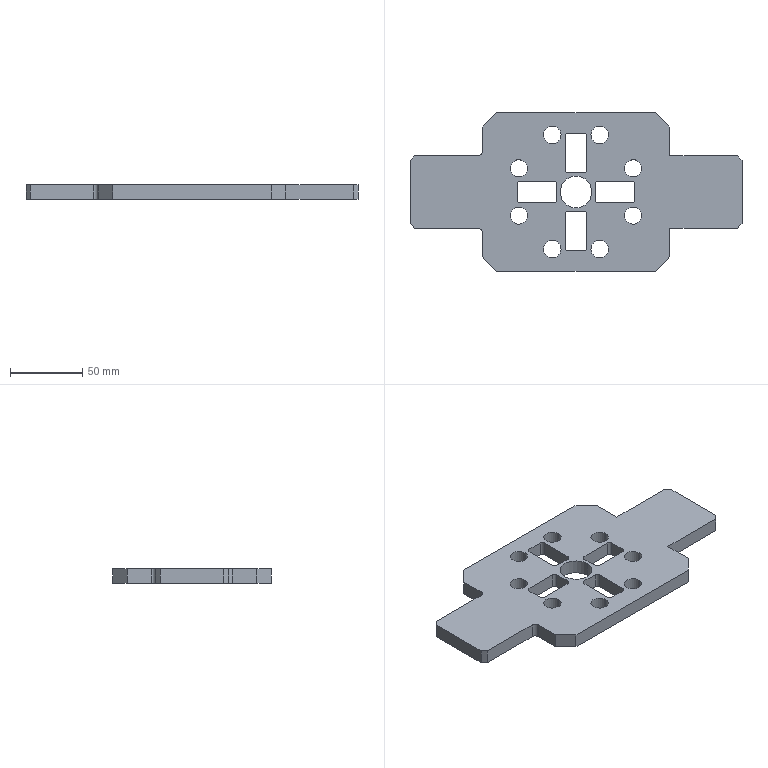Part | SolidWorks | features Cut 1, Extrusion 1, Fillet 1, ICE 1 | 1 solid | 74 faces | box 230 x 110 x 10 mm | volume 161829 mm3 | plane 38 | cylinder 36 | commonest cylinder face diameters 4 x16 12 x16 6 x2 22 x2